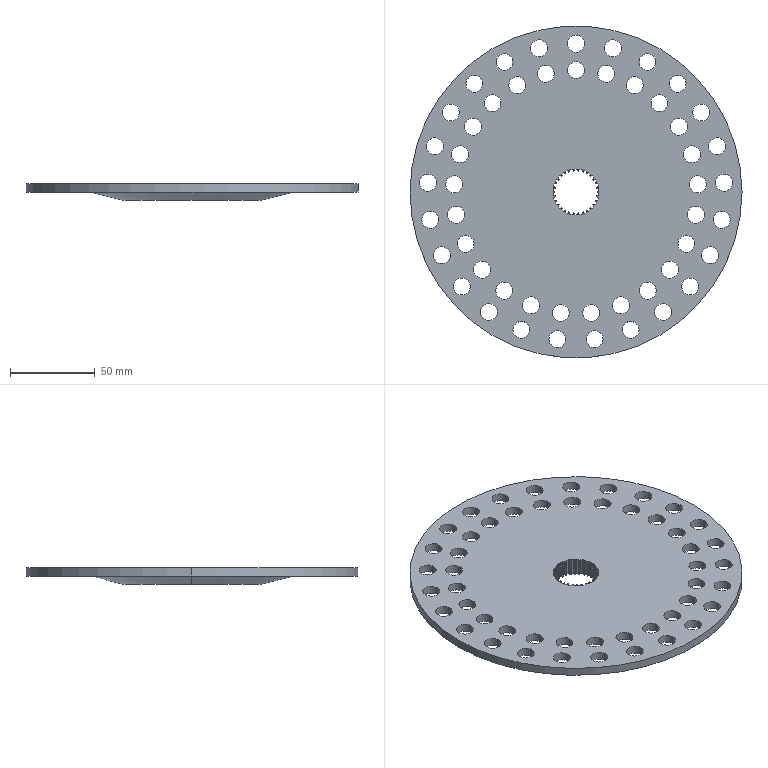Part | SolidWorks | features ICE 3, Blend 1, CirPattern 1, Extrusion 1 | 1 solid | 302 faces | box 196 x 196 x 10 mm | volume 165832 mm3 | cylinder 207 | plane 93 | cone 2 | commonest cylinder face diameters 10 x100 0.8 x74 25 x31 196 x2